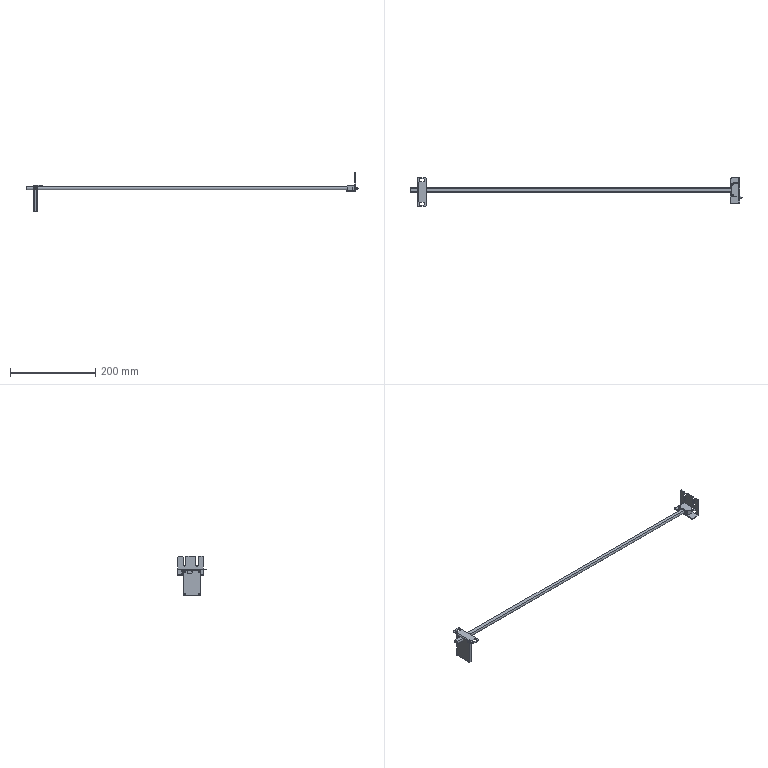Part | SolidWorks | 4 solids | 215 faces | box 779.985 x 68 x 92.8 mm | volume 89930 mm3 | plane 149 | cylinder 66 | commonest cylinder face diameters 6 x12 3.5 x9 2.5 x8 4 x8 2.6 x4 3 x4